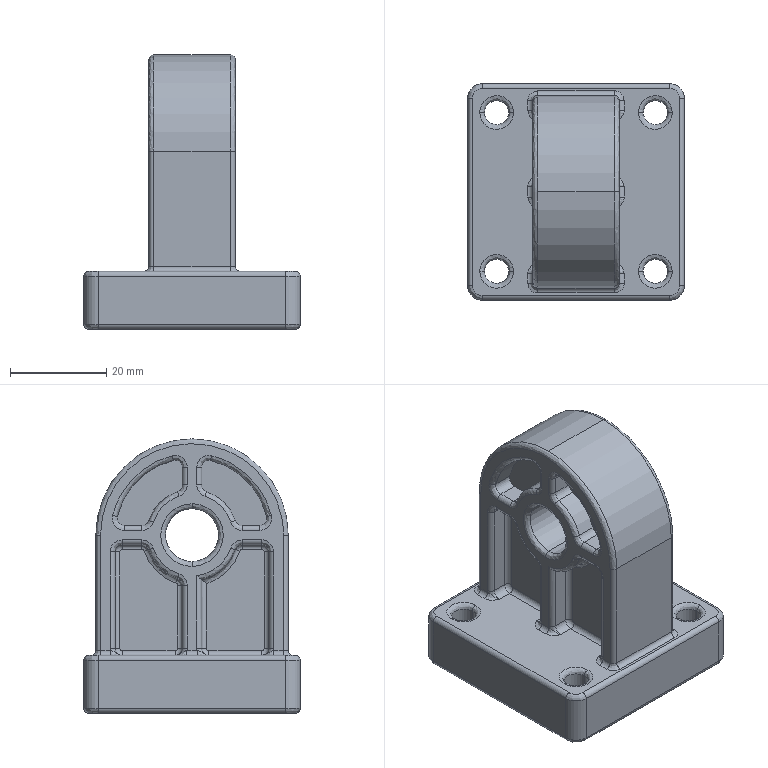Part | SolidWorks | features BaseBody 1 | 1 solid | 313 faces | box 45 x 45 x 57 mm | volume 34265 mm3 | cylinder 135 | spline 115 | plane 43 | torus 12 | cone 8 | commonest cylinder face diameters 2 x64 3 x37 5 x8 19 x8 14.05 x6 6 x4